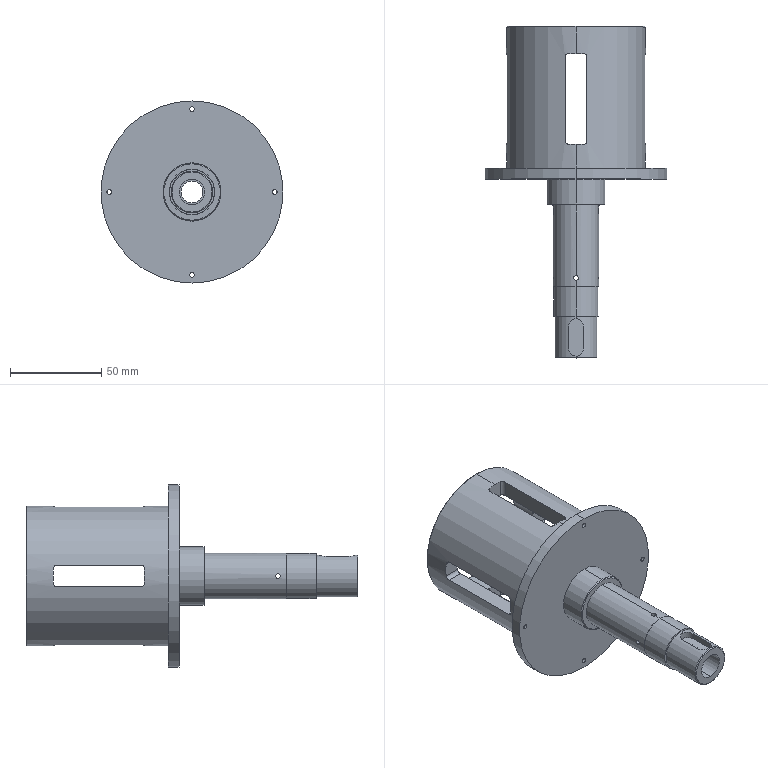Part | STEP file | ND25021-01-JDKM-12-GJ | 1 solid | 104 faces | box 100 x 182.2 x 100 mm | volume 205622 mm3 | cylinder 60 | plane 28 | cone 16 | commonest cylinder face diameters 2.5 x16 4 x16 3.3 x8 8 x2 12 x2 14 x2